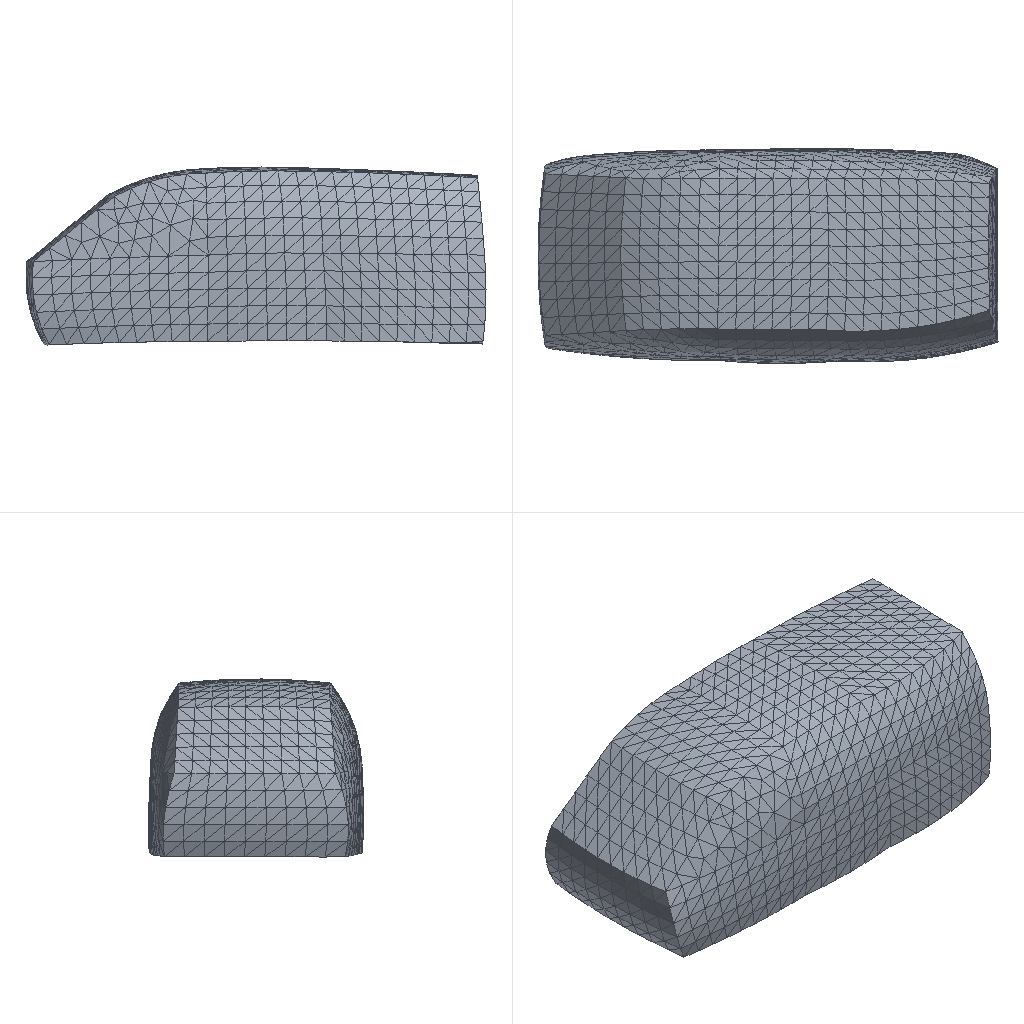Simulation study | abaqus
Set-up summary:
category,name,step,type,value,unit,region
solver,abaqus
solver,version,,,Abaqus/Standard 2020
units,not stated in the deck,,not stated
analysis,deck,,static,static
load_step,Step-1,Step-1,static
load_step,requested,,,1
mesh,nodes,,,19168
mesh,elements,,,12810
element_type,C3D10,,solid,12810
load,load commands in deck,,count,6
bc,support commands in deck,,count,2
material,MATERIAL-1,,in results
check,setup vs results,,match,"per instance, exact: element labels, types and connectivity; labels of the nodes the elements use; coordinates of those nodes at SINGLE_PRECISION in 1 of 1 instance(s)"
Abaqus input file, long lists of numbers shortened:
*Heading
** Job name: Job-2-another Model name: Model-2-Copy
** Generated by: Abaqus/CAE 2020
*Preprint, echo=NO, model=NO, history=NO, contact=NO
**
** PARTS
**
*Part, name=car2
*Node
      1,   2.277, -0.768,  0.6194
      2,   2.255,  0.7721,  0.6273
** (19166 more lines like these left out)
*Element, type=C3D10
    1,  1030,  1031,  1032,  1033,  2669,  2668,  2667,  2671,  2670,  2672
    2,  1030,  1031,  1034,  1035,  2669,  2674,  2673,  2676,  2675,  2677
** (12808 more lines like these left out)
*Nset, nset=Set-2, generate
     1,  19168,      1
*Elset, elset=Set-2, generate
     1,  12810,      1
*Nset, nset=Set-5, generate
     1,  19168,      1
*Elset, elset=Set-5, generate
     1,  12810,      1
** Section: Section-2
*Solid Section, elset=Set-5, material=Material-1
,
*End Part
**
**
** ASSEMBLY
**
*Assembly, name=Assembly
**
*Instance, name=car2-1, part=car2
*End Instance
**
*Node
      1,  0.1382,           0.,  0.8925
*Nset, nset=Set-1, instance=car2-1
     9,    10,    11,    12,    13,    14,    15,    16,    17,    18,    19,    20,    21,    22,    23,    24
    25,    98,    99,   100,   101,   102,   103,   104,   105,   106,   107,   108,   109,   110,   111,   112
** (81 more lines like these left out)
*Elset, elset=Set-1, instance=car2-1
    23,   114,  1038,  1114,  1529,  1617,  1626,  1648,  1651,  1738,  1745,  1753,  1757,  1765,  1788,  1797
  1800,  1805,  1811,  1819,  1873,  1879,  1880,  1974,  2043,  2067,  2230,  2259,  2321,  2379,  2417,  2552
** (36 more lines like these left out)
*Nset, nset=Set-4
 1,
*Nset, nset=m_Set-2
 1,
*Nset, nset=s_Set-2, instance=car2-1
     6,     7,    66,    67,    68,    69,    70,    71,    72,    73,    90,    91,    92,    93,    94,    95
    96,    97,   415,   416,   417,   418,   419,   420,   421,   422,   423,   424,   425,   426,   427,   428
** (10 more lines like these left out)
*Elset, elset=s_Set-2, instance=car2-1
   624,  2437,  2520,  2525,  2573,  2583,  2628,  2638,  2688,  2714,  2733,  2734,  2764,  2781,  2831,  2906
  2926,  2933,  2934,  2935,  2936,  2943,  2944,  2952,  2953,  2971,  2975,  2977,  2984,  2988,  2991,  2996
** (4 more lines like these left out)
*Elset, elset=_Surf-1_S3, internal, instance=car2-1
    37,   621,  1247,  1623,  1694,  1710,  1726,  1727,  1740,  1768,  1779,  1843,  1844,  1853,  1878,  1938
  1939,  1953,  1982,  2005,  2037,  2047,  2052,  2053,  2105,  2141,  2145,  2160,  2428,  2438,  2445,  2455
** (9 more lines like these left out)
*Elset, elset=_Surf-1_S1, internal, instance=car2-1
   206,  1838,  2488,  2490,  4087,  4143,  4217,  4230,  4244,  4276,  4277,  4335,  4338,  4442,  4636,  4671
  5139,  8313,  8388,  8421,  8651,  8907, 10148, 10385, 12244
*Elset, elset=_Surf-1_S2, internal, instance=car2-1
  2149,  2463,  2667,  2674,  3178,  3186,  4038,  4111,  4156,  4167,  4222,  4279,  4301,  4327,  4330,  4334
  4337,  4682,  4706,  4727,  4746,  4749,  4774,  6312,  6315,  6335,  6337,  6367,  6384,  7683, 10131
*Elset, elset=_Surf-1_S4, internal, instance=car2-1
   227,  2402,  2444,  3792,  3800,  4738,  4864,  7661,  8914,  9914, 10388
*Surface, type=ELEMENT, name=Surf-1
_Surf-1_S3, S3
_Surf-1_S1, S1
_Surf-1_S2, S2
_Surf-1_S4, S4
*Elset, elset=_Surf-2_S4, internal, instance=car2-1
  275, 2823, 3781, 5481, 7785
*Elset, elset=_Surf-2_S2, internal, instance=car2-1
  620, 2669, 2693, 2743, 2784, 2787, 2865, 3321, 3338, 3343, 3359, 3375, 3408, 3413, 3552, 3749
 5385,
*Elset, elset=_Surf-2_S3, internal, instance=car2-1
   651,  1538,  1746,  1867,  1913,  1948,  1961,  1968,  2021,  2086,  2137,  2173,  2323,  2340,  2634,  2718
  2761,  2774,  2835,  2860,  2892,  2893,  3198,  3217,  3237,  3241,  3308,  3332,  3336,  3339,  3344,  3350
** (11 more lines like these left out)
*Elset, elset=_Surf-2_S1, internal, instance=car2-1
  2279,  2695,  2804,  2891,  3264,  3285,  3296,  3323,  3342,  3351,  3368,  4290,  4452,  4586,  5371,  5664
 10081,
*Surface, type=ELEMENT, name=Surf-2
_Surf-2_S4, S4
_Surf-2_S2, S2
_Surf-2_S3, S3
_Surf-2_S1, S1
*Elset, elset=_Surf-3_S3, internal, instance=car2-1
   183,   244,   394,   402,   418,   462,   605,   711,  1380,  1658,  1792,  1809,  1870,  1875,  1898,  2668
  2737,  2905,  3628,  3661,  3763,  3770,  4012,  4037,  4060,  4069,  4100,  4179,  4307,  4384,  4436,  4717
** (19 more lines like these left out)
*Elset, elset=_Surf-3_S1, internal, instance=car2-1
  1096,  1789,  5099,  6614,  7004,  7390,  7574,  7576,  8743,  9783, 10339, 12099
*Elset, elset=_Surf-3_S2, internal, instance=car2-1
  4969,  5683,  6180,  6387,  6416,  6429,  6477,  6696,  6753,  6811,  7032,  7588,  8071, 11282
*Elset, elset=_Surf-3_S4, internal, instance=car2-1
  4695,  6589,  6637,  6698,  6706,  6834,  7137,  7160,  7466,  8594, 10905, 11159
*Surface, type=ELEMENT, name=Surf-3
_Surf-3_S3, S3
_Surf-3_S1, S1
_Surf-3_S2, S2
_Surf-3_S4, S4
*Elset, elset=_Surf-4_S4, internal, instance=car2-1
    66,    75,  1999,  4081,  7273, 10309, 12155
*Elset, elset=_Surf-4_S3, internal, instance=car2-1
  1304,  1993,  2078,  2122,  2126,  2157,  2168,  2177,  2201,  2322,  2332,  2337,  3497,  3528,  3533,  3546
  3555,  3564,  3567,  3608,  3715,  3804,  3812,  3819,  3829,  3832,  3836,  3845,  3849,  3850,  3856,  3866
** (3 more lines like these left out)
*Elset, elset=_Surf-4_S1, internal, instance=car2-1
 2250, 2271, 3498
*Elset, elset=_Surf-4_S2, internal, instance=car2-1
 3811, 3823, 3827
*Surface, type=ELEMENT, name=Surf-4
_Surf-4_S4, S4
_Surf-4_S3, S3
_Surf-4_S2, S2
_Surf-4_S1, S1
*Elset, elset=_Surf-5_S3, internal, instance=car2-1
    19,    43,   108,   113,   207,   321,   360,   401,  1280,  1616,  1620,  1636,  1642,  1646,  1657,  1660
  1663,  1666,  1667,  1684,  1695,  1701,  1707,  1717,  1718,  1720,  1721,  1722,  1736,  1737,  1750,  1752
** (23 more lines like these left out)
*Elset, elset=_Surf-5_S2, internal, instance=car2-1
  110, 2305, 2460, 2920, 3494, 4439, 4467, 4492, 4734, 5050, 5346
*Elset, elset=_Surf-5_S1, internal, instance=car2-1
 2149, 3193, 3403, 3800, 3836, 3932, 4441, 4468, 4493, 5369, 8239
*Elset, elset=_Surf-5_S4, internal, instance=car2-1
    96,  2120,  2199,  2204,  2302,  4641,  5439,  9193,  9399, 10072, 10656
*Surface, type=ELEMENT, name=Surf-5
_Surf-5_S3, S3
_Surf-5_S2, S2
_Surf-5_S4, S4
_Surf-5_S1, S1
*Surface, type=NODE, name=s_Set-2_CNS_, internal
s_Set-2, 1.
** Constraint: Constraint-1
*Coupling, constraint name=Constraint-1, ref node=m_Set-2, surface=s_Set-2_CNS_
*Kinematic
*End Assembly
*Amplitude, name=Amp-1, definition=PERIODIC
1,            710.,              0.,              0.
           1.03,              0.
**
** MATERIALS
**
*Material, name=Material-1
*Density
7890.,
*Elastic
 2.1e+11, 0.3
**
** BOUNDARY CONDITIONS
**
** Name: BC-1 Type: 对称/反对称/完全固定
*Boundary
Set-1, ENCASTRE
** ----------------------------------------------------------------
**
** STEP: Step-1
**
*Step, name=Step-1, nlgeom=YES, inc=1000
*Static, stabilize=0.0002, allsdtol=0.05, continue=NO
0.001, 0.1, 1e-06, 0.1
**
** BOUNDARY CONDITIONS
**
** Name: BC-2 Type: 速度/角速度
*Boundary, amplitude=Amp-1, type=VELOCITY
Set-4, 1, 1, 1.
**
** LOADS
**
** Name: Load-1   Type: Pressure
*Dsload
Surf-1, P, 0.037
** Name: Load-2   Type: Pressure
*Dsload
Surf-2, P, 0.037
** Name: Load-3   Type: Pressure
*Dsload
Surf-3, P, 0.037
** Name: Load-4   Type: Pressure
*Dsload
Surf-4, P, 0.037
** Name: Load-5   Type: Pressure
*Dsload
Surf-5, P, 0.037
**
** OUTPUT REQUESTS
**
*Restart, write, frequency=0
**
** FIELD OUTPUT: F-Output-1
**
*Output, field
*Node Output
CF, RF, U, V
*Element Output, directions=YES
E, LE, MISES, P, PE, PEEQ, PEMAG, S, SF
*Contact Output
CDISP, CSTRESS
**
** HISTORY OUTPUT: H-Output-1
**
*Output, history, variable=PRESELECT, frequency=10
*End Step
Results summary:
result,step,,completed,increments=12 time=0.1/0.1
result,analysis,,,static
result,last_loadstep,,,1
result,primary field,,,U
result,reaction total,,FX,423936.833,model units
result,reaction total,,FY,253.327,model units
result,reaction total,,FZ,79519.543,model units